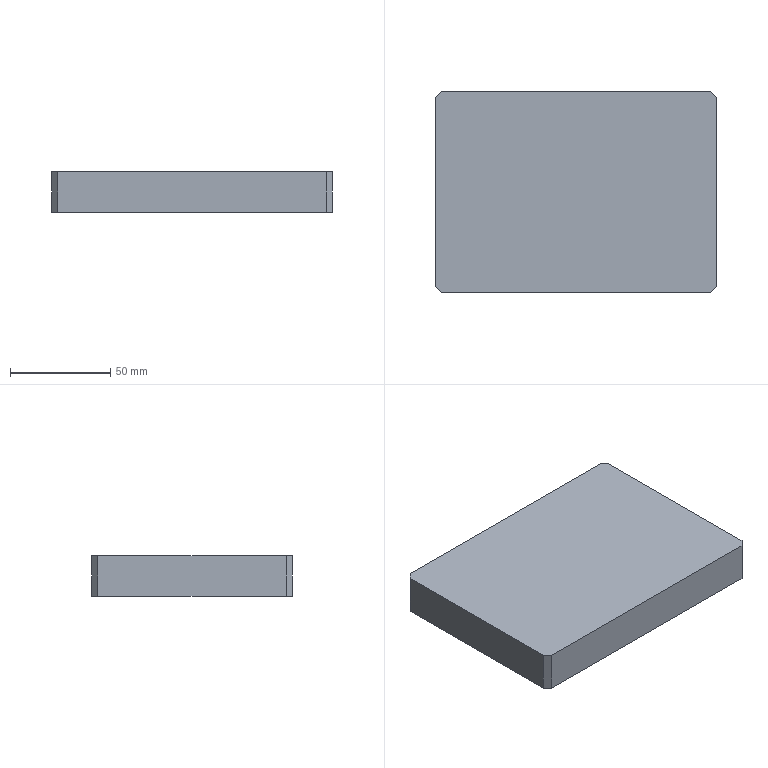Part | STEP file | 001-001-Foma caster mounting plate | 1 solid | 10 faces | box 140 x 100 x 20 mm | volume 279640 mm3 | plane 10
STEP:
#1=CARTESIAN_POINT('',(0.,0.,0.));
#2=DIRECTION('',(0.,0.,1.));
#3=DIRECTION('',(1.,0.,0.));
#4=AXIS2_PLACEMENT_3D('',#1,#2,#3);
#5=CARTESIAN_POINT('',(710.,-373.,0.));
#6=VERTEX_POINT('',#5);
#7=CARTESIAN_POINT('',(710.,-467.,0.));
#8=VERTEX_POINT('',#7);
#9=CARTESIAN_POINT('',(710.,-370.,0.));
#10=DIRECTION('',(0.,-1.,0.));
#11=VECTOR('',#10,1.);
#12=LINE('',#9,#11);
#13=CARTESIAN_POINT('',(710.,-370.,20.));
#14=DIRECTION('',(1.,0.,0.));
#15=DIRECTION('',(0.,1.,0.));
#16=AXIS2_PLACEMENT_3D('',#13,#14,#15);
#17=PLANE('',#16);
#18=CARTESIAN_POINT('',(0.,-20.));
#19=DIRECTION('',(-1.,0.));
#20=VECTOR('',#19,1.);
#21=LINE('',#18,#20);
#22=(GEOMETRIC_REPRESENTATION_CONTEXT(2)PARAMETRIC_REPRESENTATION_CONTEXT()REPRESENTATION_CONTEXT('',''));
#23=DEFINITIONAL_REPRESENTATION('',(#21),#22);
#24=PCURVE('',#17,#23);
#25=CARTESIAN_POINT('',(0.,0.,0.));
#26=DIRECTION('',(0.,0.,1.));
#27=DIRECTION('',(1.,0.,0.));
#28=AXIS2_PLACEMENT_3D('',#25,#26,#27);
#29=PLANE('',#28);
#30=CARTESIAN_POINT('',(710.,-370.));
#31=DIRECTION('',(0.,-1.));
#32=VECTOR('',#31,1.);
#33=LINE('',#30,#32);
#34=(GEOMETRIC_REPRESENTATION_CONTEXT(2)PARAMETRIC_REPRESENTATION_CONTEXT()REPRESENTATION_CONTEXT('',''));
#35=DEFINITIONAL_REPRESENTATION('',(#33),#34);
#36=PCURVE('',#29,#35);
#37=SURFACE_CURVE('',#12,(#24,#36),.PCURVE_S1.);
#38=EDGE_CURVE('',#6,#8,#37,.T.);
#39=ORIENTED_EDGE('',*,*,#38,.T.);
#40=CARTESIAN_POINT('',(710.,-467.,20.));
#41=VERTEX_POINT('',#40);
#42=CARTESIAN_POINT('',(710.,-467.,20.));
#43=DIRECTION('',(0.,0.,1.));
#44=VECTOR('',#43,1.);
#45=LINE('',#42,#44);
#46=CARTESIAN_POINT('',(-97.,0.));
#47=DIRECTION('',(0.,1.));
#48=VECTOR('',#47,1.);
#49=LINE('',#46,#48);
#50=(GEOMETRIC_REPRESENTATION_CONTEXT(2)PARAMETRIC_REPRESENTATION_CONTEXT()REPRESENTATION_CONTEXT('',''));
#51=DEFINITIONAL_REPRESENTATION('',(#49),#50);
#52=PCURVE('',#17,#51);
#53=CARTESIAN_POINT('',(713.,-470.,20.));
#54=DIRECTION('',(0.7071,0.7071,0.));
#55=DIRECTION('',(0.,0.,-1.));
#56=AXIS2_PLACEMENT_3D('',#53,#54,#55);
#57=PLANE('',#56);
#58=CARTESIAN_POINT('',(0.,4.243));
#59=DIRECTION('',(-1.,0.));
#60=VECTOR('',#59,1.);
#61=LINE('',#58,#60);
#62=(GEOMETRIC_REPRESENTATION_CONTEXT(2)PARAMETRIC_REPRESENTATION_CONTEXT()REPRESENTATION_CONTEXT('',''));
#63=DEFINITIONAL_REPRESENTATION('',(#61),#62);
#64=PCURVE('',#57,#63);
#65=SURFACE_CURVE('',#45,(#52,#64),.PCURVE_S1.);
#66=EDGE_CURVE('',#8,#41,#65,.T.);
#67=ORIENTED_EDGE('',*,*,#66,.T.);
#68=CARTESIAN_POINT('',(710.,-373.,20.));
#69=VERTEX_POINT('',#68);
#70=CARTESIAN_POINT('',(710.,-370.,20.));
#71=DIRECTION('',(0.,-1.,0.));
#72=VECTOR('',#71,1.);
#73=LINE('',#70,#72);
#74=CARTESIAN_POINT('',(0.,0.));
#75=DIRECTION('',(-1.,0.));
#76=VECTOR('',#75,1.);
#77=LINE('',#74,#76);
#78=(GEOMETRIC_REPRESENTATION_CONTEXT(2)PARAMETRIC_REPRESENTATION_CONTEXT()REPRESENTATION_CONTEXT('',''));
#79=DEFINITIONAL_REPRESENTATION('',(#77),#78);
#80=PCURVE('',#17,#79);
#81=CARTESIAN_POINT('',(0.,0.,20.));
#82=DIRECTION('',(0.,0.,1.));
#83=DIRECTION('',(1.,0.,0.));
#84=AXIS2_PLACEMENT_3D('',#81,#82,#83);
#85=PLANE('',#84);
#86=CARTESIAN_POINT('',(710.,-370.));
#87=DIRECTION('',(0.,-1.));
#88=VECTOR('',#87,1.);
#89=LINE('',#86,#88);
#90=(GEOMETRIC_REPRESENTATION_CONTEXT(2)PARAMETRIC_REPRESENTATION_CONTEXT()REPRESENTATION_CONTEXT('',''));
#91=DEFINITIONAL_REPRESENTATION('',(#89),#90);
#92=PCURVE('',#85,#91);
#93=SURFACE_CURVE('',#73,(#80,#92),.PCURVE_S1.);
#94=EDGE_CURVE('',#69,#41,#93,.T.);
#95=ORIENTED_EDGE('',*,*,#94,.F.);
#96=CARTESIAN_POINT('',(710.,-373.,20.));
#97=DIRECTION('',(0.,0.,-1.));
#98=VECTOR('',#97,1.);
#99=LINE('',#96,#98);
#100=CARTESIAN_POINT('',(-3.,0.));
#101=DIRECTION('',(0.,-1.));
#102=VECTOR('',#101,1.);
#103=LINE('',#100,#102);
#104=(GEOMETRIC_REPRESENTATION_CONTEXT(2)PARAMETRIC_REPRESENTATION_CONTEXT()REPRESENTATION_CONTEXT('',''));
#105=DEFINITIONAL_REPRESENTATION('',(#103),#104);
#106=PCURVE('',#17,#105);
#107=CARTESIAN_POINT('',(710.,-373.,20.));
#108=DIRECTION('',(0.7071,-0.7071,0.));
#109=DIRECTION('',(0.,0.,-1.));
#110=AXIS2_PLACEMENT_3D('',#107,#108,#109);
#111=PLANE('',#110);
#112=CARTESIAN_POINT('',(0.,0.));
#113=DIRECTION('',(1.,0.));
#114=VECTOR('',#113,1.);
#115=LINE('',#112,#114);
#116=(GEOMETRIC_REPRESENTATION_CONTEXT(2)PARAMETRIC_REPRESENTATION_CONTEXT()REPRESENTATION_CONTEXT('',''));
#117=DEFINITIONAL_REPRESENTATION('',(#115),#116);
#118=PCURVE('',#111,#117);
#119=SURFACE_CURVE('',#99,(#106,#118),.PCURVE_S1.);
#120=EDGE_CURVE('',#69,#6,#119,.T.);
#121=ORIENTED_EDGE('',*,*,#120,.T.);
#122=EDGE_LOOP('',(#39,#67,#95,#121));
#123=FACE_BOUND('',#122,.T.);
#124=ADVANCED_FACE('',(#123),#17,.F.);
#125=CARTESIAN_POINT('',(713.,-470.,0.));
#126=VERTEX_POINT('',#125);
#127=CARTESIAN_POINT('',(847.,-470.,0.));
#128=VERTEX_POINT('',#127);
#129=CARTESIAN_POINT('',(710.,-470.,0.));
#130=DIRECTION('',(1.,0.,0.));
#131=VECTOR('',#130,1.);
#132=LINE('',#129,#131);
#133=CARTESIAN_POINT('',(710.,-470.,20.));
#134=DIRECTION('',(0.,1.,0.));
#135=DIRECTION('',(0.,0.,1.));
#136=AXIS2_PLACEMENT_3D('',#133,#134,#135);
#137=PLANE('',#136);
#138=CARTESIAN_POINT('',(-20.,0.));
#139=DIRECTION('',(0.,1.));
#140=VECTOR('',#139,1.);
#141=LINE('',#138,#140);
#142=(GEOMETRIC_REPRESENTATION_CONTEXT(2)PARAMETRIC_REPRESENTATION_CONTEXT()REPRESENTATION_CONTEXT('',''));
#143=DEFINITIONAL_REPRESENTATION('',(#141),#142);
#144=PCURVE('',#137,#143);
#145=CARTESIAN_POINT('',(710.,-470.));
#146=DIRECTION('',(1.,0.));
#147=VECTOR('',#146,1.);
#148=LINE('',#145,#147);
#149=(GEOMETRIC_REPRESENTATION_CONTEXT(2)PARAMETRIC_REPRESENTATION_CONTEXT()REPRESENTATION_CONTEXT('',''));
#150=DEFINITIONAL_REPRESENTATION('',(#148),#149);
#151=PCURVE('',#29,#150);
#152=SURFACE_CURVE('',#132,(#144,#151),.PCURVE_S1.);
#153=EDGE_CURVE('',#126,#128,#152,.T.);
#154=ORIENTED_EDGE('',*,*,#153,.T.);
#155=CARTESIAN_POINT('',(847.,-470.,20.));
#156=VERTEX_POINT('',#155);
#157=CARTESIAN_POINT('',(847.,-470.,20.));
#158=DIRECTION('',(0.,0.,1.));
#159=VECTOR('',#158,1.);
#160=LINE('',#157,#159);
#161=CARTESIAN_POINT('',(0.,137.));
#162=DIRECTION('',(1.,0.));
#163=VECTOR('',#162,1.);
#164=LINE('',#161,#163);
#165=(GEOMETRIC_REPRESENTATION_CONTEXT(2)PARAMETRIC_REPRESENTATION_CONTEXT()REPRESENTATION_CONTEXT('',''));
#166=DEFINITIONAL_REPRESENTATION('',(#164),#165);
#167=PCURVE('',#137,#166);
#168=CARTESIAN_POINT('',(850.,-467.,20.));
#169=DIRECTION('',(-0.7071,0.7071,0.));
#170=DIRECTION('',(0.,0.,-1.));
#171=AXIS2_PLACEMENT_3D('',#168,#169,#170);
#172=PLANE('',#171);
#173=CARTESIAN_POINT('',(0.,4.243));
#174=DIRECTION('',(-1.,0.));
#175=VECTOR('',#174,1.);
#176=LINE('',#173,#175);
#177=(GEOMETRIC_REPRESENTATION_CONTEXT(2)PARAMETRIC_REPRESENTATION_CONTEXT()REPRESENTATION_CONTEXT('',''));
#178=DEFINITIONAL_REPRESENTATION('',(#176),#177);
#179=PCURVE('',#172,#178);
#180=SURFACE_CURVE('',#160,(#167,#179),.PCURVE_S1.);
#181=EDGE_CURVE('',#128,#156,#180,.T.);
#182=ORIENTED_EDGE('',*,*,#181,.T.);
#183=CARTESIAN_POINT('',(713.,-470.,20.));
#184=VERTEX_POINT('',#183);
#185=CARTESIAN_POINT('',(710.,-470.,20.));
#186=DIRECTION('',(1.,0.,0.));
#187=VECTOR('',#186,1.);
#188=LINE('',#185,#187);
#189=CARTESIAN_POINT('',(0.,0.));
#190=DIRECTION('',(0.,1.));
#191=VECTOR('',#190,1.);
#192=LINE('',#189,#191);
#193=(GEOMETRIC_REPRESENTATION_CONTEXT(2)PARAMETRIC_REPRESENTATION_CONTEXT()REPRESENTATION_CONTEXT('',''));
#194=DEFINITIONAL_REPRESENTATION('',(#192),#193);
#195=PCURVE('',#137,#194);
#196=CARTESIAN_POINT('',(710.,-470.));
#197=DIRECTION('',(1.,0.));
#198=VECTOR('',#197,1.);
#199=LINE('',#196,#198);
#200=(GEOMETRIC_REPRESENTATION_CONTEXT(2)PARAMETRIC_REPRESENTATION_CONTEXT()REPRESENTATION_CONTEXT('',''));
#201=DEFINITIONAL_REPRESENTATION('',(#199),#200);
#202=PCURVE('',#85,#201);
#203=SURFACE_CURVE('',#188,(#195,#202),.PCURVE_S1.);
#204=EDGE_CURVE('',#184,#156,#203,.T.);
#205=ORIENTED_EDGE('',*,*,#204,.F.);
#206=CARTESIAN_POINT('',(713.,-470.,20.));
#207=DIRECTION('',(0.,0.,-1.));
#208=VECTOR('',#207,1.);
#209=LINE('',#206,#208);
#210=CARTESIAN_POINT('',(0.,3.));
#211=DIRECTION('',(-1.,0.));
#212=VECTOR('',#211,1.);
#213=LINE('',#210,#212);
#214=(GEOMETRIC_REPRESENTATION_CONTEXT(2)PARAMETRIC_REPRESENTATION_CONTEXT()REPRESENTATION_CONTEXT('',''));
#215=DEFINITIONAL_REPRESENTATION('',(#213),#214);
#216=PCURVE('',#137,#215);
#217=CARTESIAN_POINT('',(0.,0.));
#218=DIRECTION('',(1.,0.));
#219=VECTOR('',#218,1.);
#220=LINE('',#217,#219);
#221=(GEOMETRIC_REPRESENTATION_CONTEXT(2)PARAMETRIC_REPRESENTATION_CONTEXT()REPRESENTATION_CONTEXT('',''));
#222=DEFINITIONAL_REPRESENTATION('',(#220),#221);
#223=PCURVE('',#57,#222);
#224=SURFACE_CURVE('',#209,(#216,#223),.PCURVE_S1.);
#225=EDGE_CURVE('',#184,#126,#224,.T.);
#226=ORIENTED_EDGE('',*,*,#225,.T.);
#227=EDGE_LOOP('',(#154,#182,#205,#226));
#228=FACE_BOUND('',#227,.T.);
#229=ADVANCED_FACE('',(#228),#137,.F.);
#230=CARTESIAN_POINT('',(850.,-467.,0.));
#231=VERTEX_POINT('',#230);
#232=CARTESIAN_POINT('',(850.,-373.,0.));
#233=VERTEX_POINT('',#232);
#234=CARTESIAN_POINT('',(850.,-370.,0.));
#235=DIRECTION('',(0.,1.,0.));
#236=VECTOR('',#235,1.);
#237=LINE('',#234,#236);
#238=CARTESIAN_POINT('',(850.,-370.,20.));
#239=DIRECTION('',(-1.,0.,0.));
#240=DIRECTION('',(0.,0.,1.));
#241=AXIS2_PLACEMENT_3D('',#238,#239,#240);
#242=PLANE('',#241);
#243=CARTESIAN_POINT('',(-20.,0.));
#244=DIRECTION('',(0.,1.));
#245=VECTOR('',#244,1.);
#246=LINE('',#243,#245);
#247=(GEOMETRIC_REPRESENTATION_CONTEXT(2)PARAMETRIC_REPRESENTATION_CONTEXT()REPRESENTATION_CONTEXT('',''));
#248=DEFINITIONAL_REPRESENTATION('',(#246),#247);
#249=PCURVE('',#242,#248);
#250=CARTESIAN_POINT('',(850.,-370.));
#251=DIRECTION('',(0.,1.));
#252=VECTOR('',#251,1.);
#253=LINE('',#250,#252);
#254=(GEOMETRIC_REPRESENTATION_CONTEXT(2)PARAMETRIC_REPRESENTATION_CONTEXT()REPRESENTATION_CONTEXT('',''));
#255=DEFINITIONAL_REPRESENTATION('',(#253),#254);
#256=PCURVE('',#29,#255);
#257=SURFACE_CURVE('',#237,(#249,#256),.PCURVE_S1.);
#258=EDGE_CURVE('',#231,#233,#257,.T.);
#259=ORIENTED_EDGE('',*,*,#258,.T.);
#260=CARTESIAN_POINT('',(850.,-373.,20.));
#261=VERTEX_POINT('',#260);
#262=CARTESIAN_POINT('',(850.,-373.,20.));
#263=DIRECTION('',(0.,0.,1.));
#264=VECTOR('',#263,1.);
#265=LINE('',#262,#264);
#266=CARTESIAN_POINT('',(0.,-3.));
#267=DIRECTION('',(1.,0.));
#268=VECTOR('',#267,1.);
#269=LINE('',#266,#268);
#270=(GEOMETRIC_REPRESENTATION_CONTEXT(2)PARAMETRIC_REPRESENTATION_CONTEXT()REPRESENTATION_CONTEXT('',''));
#271=DEFINITIONAL_REPRESENTATION('',(#269),#270);
#272=PCURVE('',#242,#271);
#273=CARTESIAN_POINT('',(847.,-370.,20.));
#274=DIRECTION('',(-0.7071,-0.7071,0.));
#275=DIRECTION('',(0.,0.,-1.));
#276=AXIS2_PLACEMENT_3D('',#273,#274,#275);
#277=PLANE('',#276);
#278=CARTESIAN_POINT('',(0.,4.243));
#279=DIRECTION('',(-1.,0.));
#280=VECTOR('',#279,1.);
#281=LINE('',#278,#280);
#282=(GEOMETRIC_REPRESENTATION_CONTEXT(2)PARAMETRIC_REPRESENTATION_CONTEXT()REPRESENTATION_CONTEXT('',''));
#283=DEFINITIONAL_REPRESENTATION('',(#281),#282);
#284=PCURVE('',#277,#283);
#285=SURFACE_CURVE('',#265,(#272,#284),.PCURVE_S1.);
#286=EDGE_CURVE('',#233,#261,#285,.T.);
#287=ORIENTED_EDGE('',*,*,#286,.T.);
#288=CARTESIAN_POINT('',(850.,-467.,20.));
#289=VERTEX_POINT('',#288);
#290=CARTESIAN_POINT('',(850.,-370.,20.));
#291=DIRECTION('',(0.,1.,0.));
#292=VECTOR('',#291,1.);
#293=LINE('',#290,#292);
#294=CARTESIAN_POINT('',(0.,0.));
#295=DIRECTION('',(0.,1.));
#296=VECTOR('',#295,1.);
#297=LINE('',#294,#296);
#298=(GEOMETRIC_REPRESENTATION_CONTEXT(2)PARAMETRIC_REPRESENTATION_CONTEXT()REPRESENTATION_CONTEXT('',''));
#299=DEFINITIONAL_REPRESENTATION('',(#297),#298);
#300=PCURVE('',#242,#299);
#301=CARTESIAN_POINT('',(850.,-370.));
#302=DIRECTION('',(0.,1.));
#303=VECTOR('',#302,1.);
#304=LINE('',#301,#303);
#305=(GEOMETRIC_REPRESENTATION_CONTEXT(2)PARAMETRIC_REPRESENTATION_CONTEXT()REPRESENTATION_CONTEXT('',''));
#306=DEFINITIONAL_REPRESENTATION('',(#304),#305);
#307=PCURVE('',#85,#306);
#308=SURFACE_CURVE('',#293,(#300,#307),.PCURVE_S1.);
#309=EDGE_CURVE('',#289,#261,#308,.T.);
#310=ORIENTED_EDGE('',*,*,#309,.F.);
#311=CARTESIAN_POINT('',(850.,-467.,20.));
#312=DIRECTION('',(0.,0.,-1.));
#313=VECTOR('',#312,1.);
#314=LINE('',#311,#313);
#315=CARTESIAN_POINT('',(0.,-97.));
#316=DIRECTION('',(-1.,0.));
#317=VECTOR('',#316,1.);
#318=LINE('',#315,#317);
#319=(GEOMETRIC_REPRESENTATION_CONTEXT(2)PARAMETRIC_REPRESENTATION_CONTEXT()REPRESENTATION_CONTEXT('',''));
#320=DEFINITIONAL_REPRESENTATION('',(#318),#319);
#321=PCURVE('',#242,#320);
#322=CARTESIAN_POINT('',(0.,0.));
#323=DIRECTION('',(1.,0.));
#324=VECTOR('',#323,1.);
#325=LINE('',#322,#324);
#326=(GEOMETRIC_REPRESENTATION_CONTEXT(2)PARAMETRIC_REPRESENTATION_CONTEXT()REPRESENTATION_CONTEXT('',''));
#327=DEFINITIONAL_REPRESENTATION('',(#325),#326);
#328=PCURVE('',#172,#327);
#329=SURFACE_CURVE('',#314,(#321,#328),.PCURVE_S1.);
#330=EDGE_CURVE('',#289,#231,#329,.T.);
#331=ORIENTED_EDGE('',*,*,#330,.T.);
#332=EDGE_LOOP('',(#259,#287,#310,#331));
#333=FACE_BOUND('',#332,.T.);
#334=ADVANCED_FACE('',(#333),#242,.F.);
#335=CARTESIAN_POINT('',(847.,-370.,20.));
#336=VERTEX_POINT('',#335);
#337=CARTESIAN_POINT('',(713.,-370.,20.));
#338=VERTEX_POINT('',#337);
#339=CARTESIAN_POINT('',(710.,-370.,20.));
#340=DIRECTION('',(-1.,0.,0.));
#341=VECTOR('',#340,1.);
#342=LINE('',#339,#341);
#343=CARTESIAN_POINT('',(710.,-370.,20.));
#344=DIRECTION('',(0.,-1.,0.));
#345=DIRECTION('',(0.,0.,-1.));
#346=AXIS2_PLACEMENT_3D('',#343,#344,#345);
#347=PLANE('',#346);
#348=CARTESIAN_POINT('',(0.,0.));
#349=DIRECTION('',(0.,-1.));
#350=VECTOR('',#349,1.);
#351=LINE('',#348,#350);
#352=(GEOMETRIC_REPRESENTATION_CONTEXT(2)PARAMETRIC_REPRESENTATION_CONTEXT()REPRESENTATION_CONTEXT('',''));
#353=DEFINITIONAL_REPRESENTATION('',(#351),#352);
#354=PCURVE('',#347,#353);
#355=CARTESIAN_POINT('',(710.,-370.));
#356=DIRECTION('',(-1.,0.));
#357=VECTOR('',#356,1.);
#358=LINE('',#355,#357);
#359=(GEOMETRIC_REPRESENTATION_CONTEXT(2)PARAMETRIC_REPRESENTATION_CONTEXT()REPRESENTATION_CONTEXT('',''));
#360=DEFINITIONAL_REPRESENTATION('',(#358),#359);
#361=PCURVE('',#85,#360);
#362=SURFACE_CURVE('',#342,(#354,#361),.PCURVE_S1.);
#363=EDGE_CURVE('',#336,#338,#362,.T.);
#364=ORIENTED_EDGE('',*,*,#363,.F.);
#365=CARTESIAN_POINT('',(847.,-370.,0.));
#366=VERTEX_POINT('',#365);
#367=CARTESIAN_POINT('',(847.,-370.,20.));
#368=DIRECTION('',(0.,0.,-1.));
#369=VECTOR('',#368,1.);
#370=LINE('',#367,#369);
#371=CARTESIAN_POINT('',(0.,137.));
#372=DIRECTION('',(1.,0.));
#373=VECTOR('',#372,1.);
#374=LINE('',#371,#373);
#375=(GEOMETRIC_REPRESENTATION_CONTEXT(2)PARAMETRIC_REPRESENTATION_CONTEXT()REPRESENTATION_CONTEXT('',''));
#376=DEFINITIONAL_REPRESENTATION('',(#374),#375);
#377=PCURVE('',#347,#376);
#378=CARTESIAN_POINT('',(0.,0.));
#379=DIRECTION('',(1.,0.));
#380=VECTOR('',#379,1.);
#381=LINE('',#378,#380);
#382=(GEOMETRIC_REPRESENTATION_CONTEXT(2)PARAMETRIC_REPRESENTATION_CONTEXT()REPRESENTATION_CONTEXT('',''));
#383=DEFINITIONAL_REPRESENTATION('',(#381),#382);
#384=PCURVE('',#277,#383);
#385=SURFACE_CURVE('',#370,(#377,#384),.PCURVE_S1.);
#386=EDGE_CURVE('',#336,#366,#385,.T.);
#387=ORIENTED_EDGE('',*,*,#386,.T.);
#388=CARTESIAN_POINT('',(713.,-370.,0.));
#389=VERTEX_POINT('',#388);
#390=CARTESIAN_POINT('',(710.,-370.,0.));
#391=DIRECTION('',(-1.,0.,0.));
#392=VECTOR('',#391,1.);
#393=LINE('',#390,#392);
#394=CARTESIAN_POINT('',(20.,0.));
#395=DIRECTION('',(0.,-1.));
#396=VECTOR('',#395,1.);
#397=LINE('',#394,#396);
#398=(GEOMETRIC_REPRESENTATION_CONTEXT(2)PARAMETRIC_REPRESENTATION_CONTEXT()REPRESENTATION_CONTEXT('',''));
#399=DEFINITIONAL_REPRESENTATION('',(#397),#398);
#400=PCURVE('',#347,#399);
#401=CARTESIAN_POINT('',(710.,-370.));
#402=DIRECTION('',(-1.,0.));
#403=VECTOR('',#402,1.);
#404=LINE('',#401,#403);
#405=(GEOMETRIC_REPRESENTATION_CONTEXT(2)PARAMETRIC_REPRESENTATION_CONTEXT()REPRESENTATION_CONTEXT('',''));
#406=DEFINITIONAL_REPRESENTATION('',(#404),#405);
#407=PCURVE('',#29,#406);
#408=SURFACE_CURVE('',#393,(#400,#407),.PCURVE_S1.);
#409=EDGE_CURVE('',#366,#389,#408,.T.);
#410=ORIENTED_EDGE('',*,*,#409,.T.);
#411=CARTESIAN_POINT('',(713.,-370.,20.));
#412=DIRECTION('',(0.,0.,1.));
#413=VECTOR('',#412,1.);
#414=LINE('',#411,#413);
#415=CARTESIAN_POINT('',(0.,3.));
#416=DIRECTION('',(-1.,0.));
#417=VECTOR('',#416,1.);
#418=LINE('',#415,#417);
#419=(GEOMETRIC_REPRESENTATION_CONTEXT(2)PARAMETRIC_REPRESENTATION_CONTEXT()REPRESENTATION_CONTEXT('',''));
#420=DEFINITIONAL_REPRESENTATION('',(#418),#419);
#421=PCURVE('',#347,#420);
#422=CARTESIAN_POINT('',(0.,4.243));
#423=DIRECTION('',(-1.,0.));
#424=VECTOR('',#423,1.);
#425=LINE('',#422,#424);
#426=(GEOMETRIC_REPRESENTATION_CONTEXT(2)PARAMETRIC_REPRESENTATION_CONTEXT()REPRESENTATION_CONTEXT('',''));
#427=DEFINITIONAL_REPRESENTATION('',(#425),#426);
#428=PCURVE('',#111,#427);
#429=SURFACE_CURVE('',#414,(#421,#428),.PCURVE_S1.);
#430=EDGE_CURVE('',#389,#338,#429,.T.);
#431=ORIENTED_EDGE('',*,*,#430,.T.);
#432=EDGE_LOOP('',(#364,#387,#410,#431));
#433=FACE_BOUND('',#432,.T.);
#434=ADVANCED_FACE('',(#433),#347,.F.);
#435=ORIENTED_EDGE('',*,*,#309,.T.);
#436=CARTESIAN_POINT('',(238.5,238.5,20.));
#437=DIRECTION('',(-0.7071,0.7071,0.));
#438=VECTOR('',#437,1.);
#439=LINE('',#436,#438);
#440=CARTESIAN_POINT('',(238.5,238.5));
#441=DIRECTION('',(-0.7071,0.7071));
#442=VECTOR('',#441,1.);
#443=LINE('',#440,#442);
#444=(GEOMETRIC_REPRESENTATION_CONTEXT(2)PARAMETRIC_REPRESENTATION_CONTEXT()REPRESENTATION_CONTEXT('',''));
#445=DEFINITIONAL_REPRESENTATION('',(#443),#444);
#446=PCURVE('',#85,#445);
#447=CARTESIAN_POINT('',(0.,-860.549));
#448=DIRECTION('',(0.,-1.));
#449=VECTOR('',#448,1.);
#450=LINE('',#447,#449);
#451=(GEOMETRIC_REPRESENTATION_CONTEXT(2)PARAMETRIC_REPRESENTATION_CONTEXT()REPRESENTATION_CONTEXT('',''));
#452=DEFINITIONAL_REPRESENTATION('',(#450),#451);
#453=PCURVE('',#277,#452);
#454=SURFACE_CURVE('',#439,(#446,#453),.PCURVE_S1.);
#455=EDGE_CURVE('',#261,#336,#454,.T.);
#456=ORIENTED_EDGE('',*,*,#455,.T.);
#457=ORIENTED_EDGE('',*,*,#363,.T.);
#458=CARTESIAN_POINT('',(541.5,-541.5,20.));
#459=DIRECTION('',(-0.7071,-0.7071,0.));
#460=VECTOR('',#459,1.);
#461=LINE('',#458,#460);
#462=CARTESIAN_POINT('',(541.5,-541.5));
#463=DIRECTION('',(-0.7071,-0.7071));
#464=VECTOR('',#463,1.);
#465=LINE('',#462,#464);
#466=(GEOMETRIC_REPRESENTATION_CONTEXT(2)PARAMETRIC_REPRESENTATION_CONTEXT()REPRESENTATION_CONTEXT('',''));
#467=DEFINITIONAL_REPRESENTATION('',(#465),#466);
#468=PCURVE('',#85,#467);
#469=CARTESIAN_POINT('',(0.,-238.295));
#470=DIRECTION('',(0.,-1.));
#471=VECTOR('',#470,1.);
#472=LINE('',#469,#471);
#473=(GEOMETRIC_REPRESENTATION_CONTEXT(2)PARAMETRIC_REPRESENTATION_CONTEXT()REPRESENTATION_CONTEXT('',''));
#474=DEFINITIONAL_REPRESENTATION('',(#472),#473);
#475=PCURVE('',#111,#474);
#476=SURFACE_CURVE('',#461,(#468,#475),.PCURVE_S1.);
#477=EDGE_CURVE('',#338,#69,#476,.T.);
#478=ORIENTED_EDGE('',*,*,#477,.T.);
#479=ORIENTED_EDGE('',*,*,#94,.T.);
#480=CARTESIAN_POINT('',(121.5,121.5,20.));
#481=DIRECTION('',(0.7071,-0.7071,0.));
#482=VECTOR('',#481,1.);
#483=LINE('',#480,#482);
#484=CARTESIAN_POINT('',(121.5,121.5));
#485=DIRECTION('',(0.7071,-0.7071));
#486=VECTOR('',#485,1.);
#487=LINE('',#484,#486);
#488=(GEOMETRIC_REPRESENTATION_CONTEXT(2)PARAMETRIC_REPRESENTATION_CONTEXT()REPRESENTATION_CONTEXT('',''));
#489=DEFINITIONAL_REPRESENTATION('',(#487),#488);
#490=PCURVE('',#85,#489);
#491=CARTESIAN_POINT('',(0.,836.507));
#492=DIRECTION('',(0.,-1.));
#493=VECTOR('',#492,1.);
#494=LINE('',#491,#493);
#495=(GEOMETRIC_REPRESENTATION_CONTEXT(2)PARAMETRIC_REPRESENTATION_CONTEXT()REPRESENTATION_CONTEXT('',''));
#496=DEFINITIONAL_REPRESENTATION('',(#494),#495);
#497=PCURVE('',#57,#496);
#498=SURFACE_CURVE('',#483,(#490,#497),.PCURVE_S1.);
#499=EDGE_CURVE('',#41,#184,#498,.T.);
#500=ORIENTED_EDGE('',*,*,#499,.T.);
#501=ORIENTED_EDGE('',*,*,#204,.T.);
#502=CARTESIAN_POINT('',(658.5,-658.5,20.));
#503=DIRECTION('',(0.7071,0.7071,0.));
#504=VECTOR('',#503,1.);
#505=LINE('',#502,#504);
#506=CARTESIAN_POINT('',(658.5,-658.5));
#507=DIRECTION('',(0.7071,0.7071));
#508=VECTOR('',#507,1.);
#509=LINE('',#506,#508);
#510=(GEOMETRIC_REPRESENTATION_CONTEXT(2)PARAMETRIC_REPRESENTATION_CONTEXT()REPRESENTATION_CONTEXT('',''));
#511=DEFINITIONAL_REPRESENTATION('',(#509),#510);
#512=PCURVE('',#85,#511);
#513=CARTESIAN_POINT('',(0.,270.822));
#514=DIRECTION('',(0.,-1.));
#515=VECTOR('',#514,1.);
#516=LINE('',#513,#515);
#517=(GEOMETRIC_REPRESENTATION_CONTEXT(2)PARAMETRIC_REPRESENTATION_CONTEXT()REPRESENTATION_CONTEXT('',''));
#518=DEFINITIONAL_REPRESENTATION('',(#516),#517);
#519=PCURVE('',#172,#518);
#520=SURFACE_CURVE('',#505,(#512,#519),.PCURVE_S1.);
#521=EDGE_CURVE('',#156,#289,#520,.T.);
#522=ORIENTED_EDGE('',*,*,#521,.T.);
#523=EDGE_LOOP('',(#435,#456,#457,#478,#479,#500,#501,#522));
#524=FACE_BOUND('',#523,.T.);
#525=ADVANCED_FACE('',(#524),#85,.T.);
#526=ORIENTED_EDGE('',*,*,#409,.F.);
#527=CARTESIAN_POINT('',(847.,-370.,0.));
#528=DIRECTION('',(0.7071,-0.7071,0.));
#529=VECTOR('',#528,1.);
#530=LINE('',#527,#529);
#531=CARTESIAN_POINT('',(847.,-370.));
#532=DIRECTION('',(0.7071,-0.7071));
#533=VECTOR('',#532,1.);
#534=LINE('',#531,#533);
#535=(GEOMETRIC_REPRESENTATION_CONTEXT(2)PARAMETRIC_REPRESENTATION_CONTEXT()REPRESENTATION_CONTEXT('',''));
#536=DEFINITIONAL_REPRESENTATION('',(#534),#535);
#537=PCURVE('',#29,#536);
#538=CARTESIAN_POINT('',(20.,0.));
#539=DIRECTION('',(0.,1.));
#540=VECTOR('',#539,1.);
#541=LINE('',#538,#540);
#542=(GEOMETRIC_REPRESENTATION_CONTEXT(2)PARAMETRIC_REPRESENTATION_CONTEXT()REPRESENTATION_CONTEXT('',''));
#543=DEFINITIONAL_REPRESENTATION('',(#541),#542);
#544=PCURVE('',#277,#543);
#545=SURFACE_CURVE('',#530,(#537,#544),.PCURVE_S1.);
#546=EDGE_CURVE('',#366,#233,#545,.T.);
#547=ORIENTED_EDGE('',*,*,#546,.T.);
#548=ORIENTED_EDGE('',*,*,#258,.F.);
#549=CARTESIAN_POINT('',(850.,-467.,0.));
#550=DIRECTION('',(-0.7071,-0.7071,0.));
#551=VECTOR('',#550,1.);
#552=LINE('',#549,#551);
#553=CARTESIAN_POINT('',(850.,-467.));
#554=DIRECTION('',(-0.7071,-0.7071));
#555=VECTOR('',#554,1.);
#556=LINE('',#553,#555);
#557=(GEOMETRIC_REPRESENTATION_CONTEXT(2)PARAMETRIC_REPRESENTATION_CONTEXT()REPRESENTATION_CONTEXT('',''));
#558=DEFINITIONAL_REPRESENTATION('',(#556),#557);
#559=PCURVE('',#29,#558);
#560=CARTESIAN_POINT('',(20.,0.));
#561=DIRECTION('',(0.,1.));
#562=VECTOR('',#561,1.);
#563=LINE('',#560,#562);
#564=(GEOMETRIC_REPRESENTATION_CONTEXT(2)PARAMETRIC_REPRESENTATION_CONTEXT()REPRESENTATION_CONTEXT('',''));
#565=DEFINITIONAL_REPRESENTATION('',(#563),#564);
#566=PCURVE('',#172,#565);
#567=SURFACE_CURVE('',#552,(#559,#566),.PCURVE_S1.);
#568=EDGE_CURVE('',#231,#128,#567,.T.);
#569=ORIENTED_EDGE('',*,*,#568,.T.);
#570=ORIENTED_EDGE('',*,*,#153,.F.);
#571=CARTESIAN_POINT('',(713.,-470.,0.));
#572=DIRECTION('',(-0.7071,0.7071,0.));
#573=VECTOR('',#572,1.);
#574=LINE('',#571,#573);
#575=CARTESIAN_POINT('',(713.,-470.));
#576=DIRECTION('',(-0.7071,0.7071));
#577=VECTOR('',#576,1.);
#578=LINE('',#575,#577);
#579=(GEOMETRIC_REPRESENTATION_CONTEXT(2)PARAMETRIC_REPRESENTATION_CONTEXT()REPRESENTATION_CONTEXT('',''));
#580=DEFINITIONAL_REPRESENTATION('',(#578),#579);
#581=PCURVE('',#29,#580);
#582=CARTESIAN_POINT('',(20.,0.));
#583=DIRECTION('',(0.,1.));
#584=VECTOR('',#583,1.);
#585=LINE('',#582,#584);
#586=(GEOMETRIC_REPRESENTATION_CONTEXT(2)PARAMETRIC_REPRESENTATION_CONTEXT()REPRESENTATION_CONTEXT('',''));
#587=DEFINITIONAL_REPRESENTATION('',(#585),#586);
#588=PCURVE('',#57,#587);
#589=SURFACE_CURVE('',#574,(#581,#588),.PCURVE_S1.);
#590=EDGE_CURVE('',#126,#8,#589,.T.);
#591=ORIENTED_EDGE('',*,*,#590,.T.);
#592=ORIENTED_EDGE('',*,*,#38,.F.);
#593=CARTESIAN_POINT('',(710.,-373.,0.));
#594=DIRECTION('',(0.7071,0.7071,0.));
#595=VECTOR('',#594,1.);
#596=LINE('',#593,#595);
#597=CARTESIAN_POINT('',(710.,-373.));
#598=DIRECTION('',(0.7071,0.7071));
#599=VECTOR('',#598,1.);
#600=LINE('',#597,#599);
#601=(GEOMETRIC_REPRESENTATION_CONTEXT(2)PARAMETRIC_REPRESENTATION_CONTEXT()REPRESENTATION_CONTEXT('',''));
#602=DEFINITIONAL_REPRESENTATION('',(#600),#601);
#603=PCURVE('',#29,#602);
#604=CARTESIAN_POINT('',(20.,0.));
#605=DIRECTION('',(0.,1.));
#606=VECTOR('',#605,1.);
#607=LINE('',#604,#606);
#608=(GEOMETRIC_REPRESENTATION_CONTEXT(2)PARAMETRIC_REPRESENTATION_CONTEXT()REPRESENTATION_CONTEXT('',''));
#609=DEFINITIONAL_REPRESENTATION('',(#607),#608);
#610=PCURVE('',#111,#609);
#611=SURFACE_CURVE('',#596,(#603,#610),.PCURVE_S1.);
#612=EDGE_CURVE('',#6,#389,#611,.T.);
#613=ORIENTED_EDGE('',*,*,#612,.T.);
#614=EDGE_LOOP('',(#526,#547,#548,#569,#570,#591,#592,#613));
#615=FACE_BOUND('',#614,.T.);
#616=ADVANCED_FACE('',(#615),#29,.F.);
#617=ORIENTED_EDGE('',*,*,#455,.F.);
#618=ORIENTED_EDGE('',*,*,#286,.F.);
#619=ORIENTED_EDGE('',*,*,#546,.F.);
#620=ORIENTED_EDGE('',*,*,#386,.F.);
#621=EDGE_LOOP('',(#617,#618,#619,#620));
#622=FACE_BOUND('',#621,.T.);
#623=ADVANCED_FACE('',(#622),#277,.F.);
#624=ORIENTED_EDGE('',*,*,#521,.F.);
#625=ORIENTED_EDGE('',*,*,#181,.F.);
#626=ORIENTED_EDGE('',*,*,#568,.F.);
#627=ORIENTED_EDGE('',*,*,#330,.F.);
#628=EDGE_LOOP('',(#624,#625,#626,#627));
#629=FACE_BOUND('',#628,.T.);
#630=ADVANCED_FACE('',(#629),#172,.F.);
#631=ORIENTED_EDGE('',*,*,#499,.F.);
#632=ORIENTED_EDGE('',*,*,#66,.F.);
#633=ORIENTED_EDGE('',*,*,#590,.F.);
#634=ORIENTED_EDGE('',*,*,#225,.F.);
#635=EDGE_LOOP('',(#631,#632,#633,#634));
#636=FACE_BOUND('',#635,.T.);
#637=ADVANCED_FACE('',(#636),#57,.F.);
#638=ORIENTED_EDGE('',*,*,#477,.F.);
#639=ORIENTED_EDGE('',*,*,#430,.F.);
#640=ORIENTED_EDGE('',*,*,#612,.F.);
#641=ORIENTED_EDGE('',*,*,#120,.F.);
#642=EDGE_LOOP('',(#638,#639,#640,#641));
#643=FACE_BOUND('',#642,.T.);
#644=ADVANCED_FACE('',(#643),#111,.F.);
#645=CLOSED_SHELL('',(#124,#229,#334,#434,#525,#616,#623,#630,#637,#644));
#646=MANIFOLD_SOLID_BREP('',#645);
#647=(LENGTH_UNIT()NAMED_UNIT(*)SI_UNIT(.MILLI.,.METRE.));
#648=UNCERTAINTY_MEASURE_WITH_UNIT(LENGTH_MEASURE(0.0000001),#647,'','');
#649=(NAMED_UNIT(*)PLANE_ANGLE_UNIT()SI_UNIT($,.RADIAN.));
#650=(NAMED_UNIT(*)SI_UNIT($,.STERADIAN.)SOLID_ANGLE_UNIT());
#651=(GEOMETRIC_REPRESENTATION_CONTEXT(3)GLOBAL_UNCERTAINTY_ASSIGNED_CONTEXT((#648))GLOBAL_UNIT_ASSIGNED_CONTEXT((#647,#649,#650))REPRESENTATION_CONTEXT('',''));
#652=ADVANCED_BREP_SHAPE_REPRESENTATION('',(#4,#646),#651);